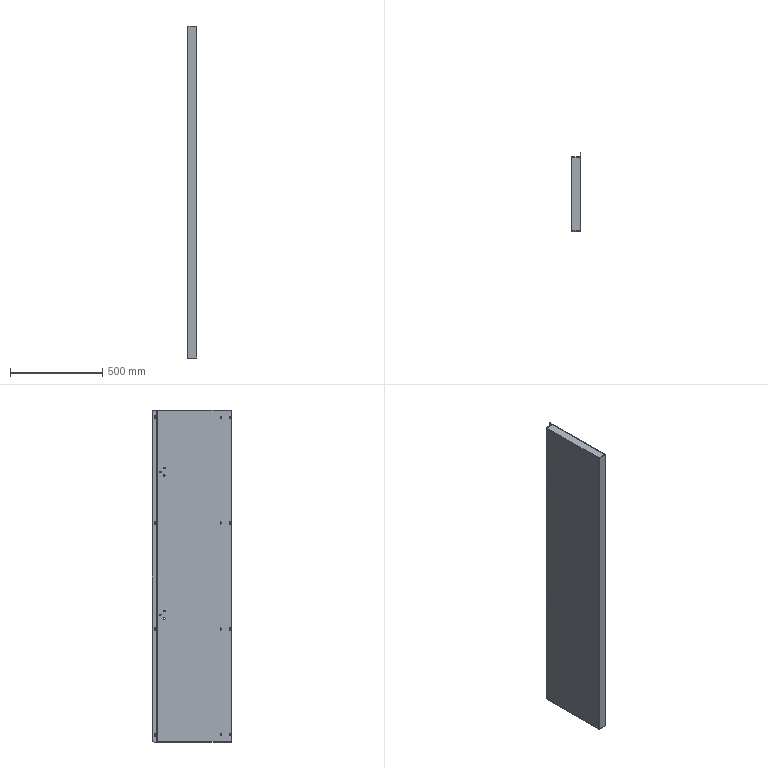Part | SolidWorks | 1 solid | 168 faces | box 50 x 430 x 1800 mm | volume 1586446 mm3 | plane 100 | cylinder 68 | commonest cylinder face diameters 6 x16 7 x12 8.5 x12 2 x9 5 x9 8 x8